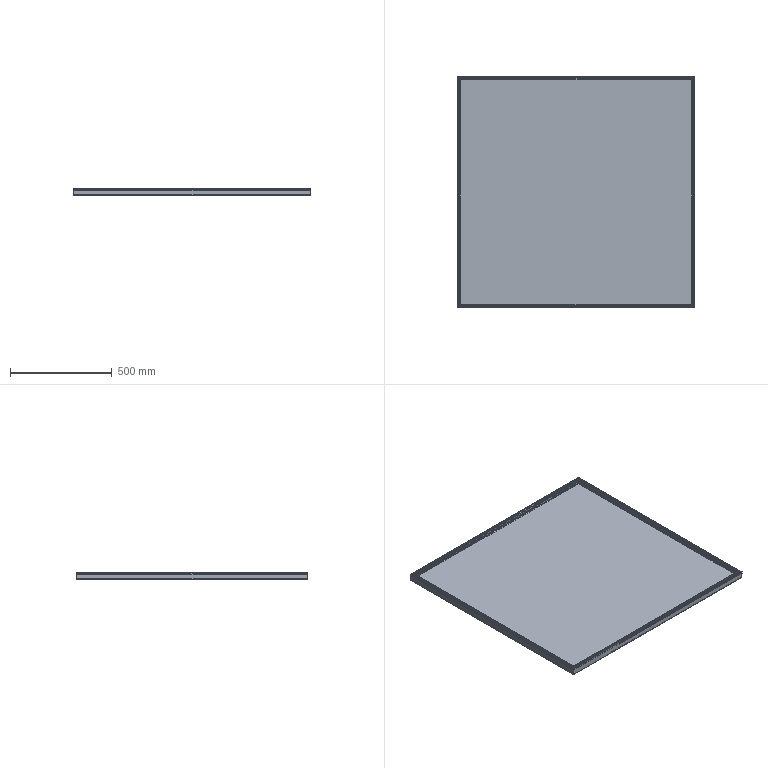Part | 5 solids | 94 faces | box 1170 x 1140 x 35 mm | volume 4589073 mm3 | plane 86 | cylinder 8 | commonest cylinder face diameters 1 x4 2 x4